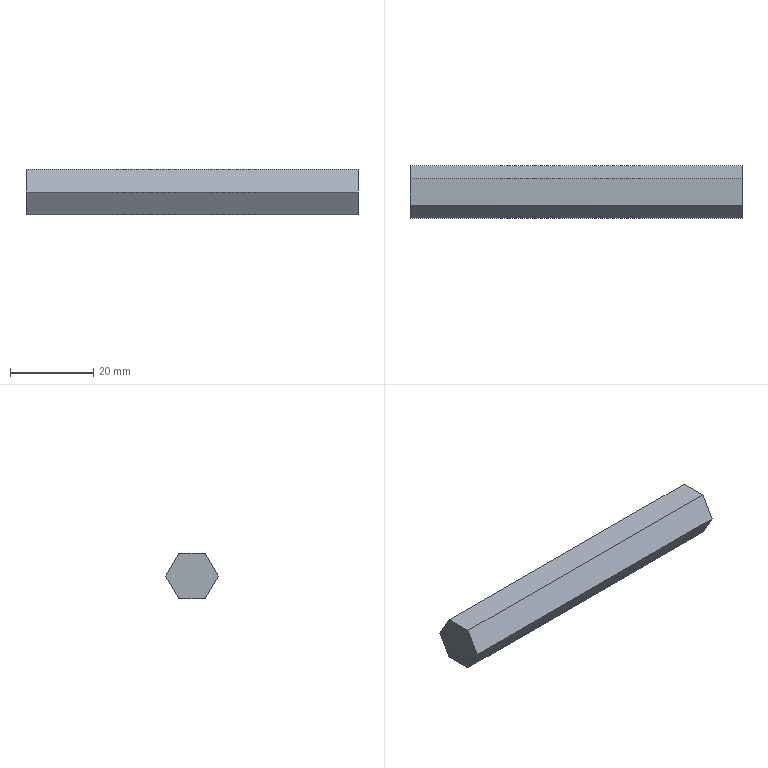Part | NX | features BREP 1 | 1 solid | 8 faces | box 80 x 12.702 x 11 mm | volume 8383 mm3 | plane 8
STEP:
#1=CARTESIAN_POINT('',(0.,-3.175,-5.5));
#2=VERTEX_POINT('',#1);
#3=CARTESIAN_POINT('',(0.,3.175,-5.5));
#4=VERTEX_POINT('',#3);
#5=CARTESIAN_POINT('',(0.,-3.175,-5.5));
#6=DIRECTION('',(0.,1.,0.));
#7=VECTOR('',#6,1000.);
#8=LINE('',#5,#7);
#9=EDGE_CURVE('',#2,#4,#8,.T.);
#10=ORIENTED_EDGE('',*,*,#9,.F.);
#11=CARTESIAN_POINT('',(0.,-6.351,0.));
#12=VERTEX_POINT('',#11);
#13=CARTESIAN_POINT('',(0.,-6.351,0.));
#14=DIRECTION('',(0.,0.5,-0.866));
#15=VECTOR('',#14,1000.);
#16=LINE('',#13,#15);
#17=EDGE_CURVE('',#12,#2,#16,.T.);
#18=ORIENTED_EDGE('',*,*,#17,.F.);
#19=CARTESIAN_POINT('',(0.,-3.175,5.5));
#20=VERTEX_POINT('',#19);
#21=CARTESIAN_POINT('',(0.,-3.175,5.5));
#22=DIRECTION('',(0.,-0.5,-0.866));
#23=VECTOR('',#22,1000.);
#24=LINE('',#21,#23);
#25=EDGE_CURVE('',#20,#12,#24,.T.);
#26=ORIENTED_EDGE('',*,*,#25,.F.);
#27=CARTESIAN_POINT('',(0.,3.175,5.5));
#28=VERTEX_POINT('',#27);
#29=CARTESIAN_POINT('',(0.,3.175,5.5));
#30=DIRECTION('',(0.,-1.,0.));
#31=VECTOR('',#30,1000.);
#32=LINE('',#29,#31);
#33=EDGE_CURVE('',#28,#20,#32,.T.);
#34=ORIENTED_EDGE('',*,*,#33,.F.);
#35=CARTESIAN_POINT('',(0.,6.351,0.));
#36=VERTEX_POINT('',#35);
#37=CARTESIAN_POINT('',(0.,6.351,0.));
#38=DIRECTION('',(0.,-0.5,0.866));
#39=VECTOR('',#38,1000.);
#40=LINE('',#37,#39);
#41=EDGE_CURVE('',#36,#28,#40,.T.);
#42=ORIENTED_EDGE('',*,*,#41,.F.);
#43=CARTESIAN_POINT('',(0.,3.175,-5.5));
#44=DIRECTION('',(0.,0.5,0.866));
#45=VECTOR('',#44,1000.);
#46=LINE('',#43,#45);
#47=EDGE_CURVE('',#4,#36,#46,.T.);
#48=ORIENTED_EDGE('',*,*,#47,.F.);
#49=EDGE_LOOP('',(#10,#18,#26,#34,#42,#48));
#50=FACE_BOUND('',#49,.T.);
#51=CARTESIAN_POINT('',(0.,0.,0.));
#52=DIRECTION('',(1.,0.,0.));
#53=DIRECTION('',(0.,1.,0.));
#54=AXIS2_PLACEMENT_3D('',#51,#52,#53);
#55=PLANE('',#54);
#56=ADVANCED_FACE('',(#50),#55,.F.);
#57=CARTESIAN_POINT('',(80.,6.351,0.));
#58=VERTEX_POINT('',#57);
#59=CARTESIAN_POINT('',(0.,6.351,0.));
#60=DIRECTION('',(1.,0.,0.));
#61=VECTOR('',#60,1000.);
#62=LINE('',#59,#61);
#63=EDGE_CURVE('',#36,#58,#62,.T.);
#64=ORIENTED_EDGE('',*,*,#63,.T.);
#65=CARTESIAN_POINT('',(80.,3.175,-5.5));
#66=VERTEX_POINT('',#65);
#67=CARTESIAN_POINT('',(80.,3.175,-5.5));
#68=DIRECTION('',(0.,0.5,0.866));
#69=VECTOR('',#68,1000.);
#70=LINE('',#67,#69);
#71=EDGE_CURVE('',#66,#58,#70,.T.);
#72=ORIENTED_EDGE('',*,*,#71,.F.);
#73=CARTESIAN_POINT('',(0.,3.175,-5.5));
#74=DIRECTION('',(1.,0.,0.));
#75=VECTOR('',#74,1000.);
#76=LINE('',#73,#75);
#77=EDGE_CURVE('',#4,#66,#76,.T.);
#78=ORIENTED_EDGE('',*,*,#77,.F.);
#79=ORIENTED_EDGE('',*,*,#47,.T.);
#80=EDGE_LOOP('',(#64,#72,#78,#79));
#81=FACE_BOUND('',#80,.T.);
#82=CARTESIAN_POINT('',(0.,3.175,-5.5));
#83=DIRECTION('',(0.,0.866,-0.5));
#84=DIRECTION('',(-1.,0.,0.));
#85=AXIS2_PLACEMENT_3D('',#82,#83,#84);
#86=PLANE('',#85);
#87=ADVANCED_FACE('',(#81),#86,.T.);
#88=ORIENTED_EDGE('',*,*,#77,.T.);
#89=CARTESIAN_POINT('',(80.,-3.175,-5.5));
#90=VERTEX_POINT('',#89);
#91=CARTESIAN_POINT('',(80.,-3.175,-5.5));
#92=DIRECTION('',(0.,1.,0.));
#93=VECTOR('',#92,1000.);
#94=LINE('',#91,#93);
#95=EDGE_CURVE('',#90,#66,#94,.T.);
#96=ORIENTED_EDGE('',*,*,#95,.F.);
#97=CARTESIAN_POINT('',(0.,-3.175,-5.5));
#98=DIRECTION('',(1.,0.,0.));
#99=VECTOR('',#98,1000.);
#100=LINE('',#97,#99);
#101=EDGE_CURVE('',#2,#90,#100,.T.);
#102=ORIENTED_EDGE('',*,*,#101,.F.);
#103=ORIENTED_EDGE('',*,*,#9,.T.);
#104=EDGE_LOOP('',(#88,#96,#102,#103));
#105=FACE_BOUND('',#104,.T.);
#106=CARTESIAN_POINT('',(0.,-3.175,-5.5));
#107=DIRECTION('',(0.,0.,-1.));
#108=DIRECTION('',(0.,-1.,0.));
#109=AXIS2_PLACEMENT_3D('',#106,#107,#108);
#110=PLANE('',#109);
#111=ADVANCED_FACE('',(#105),#110,.T.);
#112=ORIENTED_EDGE('',*,*,#101,.T.);
#113=CARTESIAN_POINT('',(80.,-6.351,0.));
#114=VERTEX_POINT('',#113);
#115=CARTESIAN_POINT('',(80.,-6.351,0.));
#116=DIRECTION('',(0.,0.5,-0.866));
#117=VECTOR('',#116,1000.);
#118=LINE('',#115,#117);
#119=EDGE_CURVE('',#114,#90,#118,.T.);
#120=ORIENTED_EDGE('',*,*,#119,.F.);
#121=CARTESIAN_POINT('',(0.,-6.351,0.));
#122=DIRECTION('',(1.,0.,0.));
#123=VECTOR('',#122,1000.);
#124=LINE('',#121,#123);
#125=EDGE_CURVE('',#12,#114,#124,.T.);
#126=ORIENTED_EDGE('',*,*,#125,.F.);
#127=ORIENTED_EDGE('',*,*,#17,.T.);
#128=EDGE_LOOP('',(#112,#120,#126,#127));
#129=FACE_BOUND('',#128,.T.);
#130=CARTESIAN_POINT('',(0.,-6.351,0.));
#131=DIRECTION('',(0.,-0.866,-0.5));
#132=DIRECTION('',(0.,0.5,-0.866));
#133=AXIS2_PLACEMENT_3D('',#130,#131,#132);
#134=PLANE('',#133);
#135=ADVANCED_FACE('',(#129),#134,.T.);
#136=ORIENTED_EDGE('',*,*,#125,.T.);
#137=CARTESIAN_POINT('',(80.,-3.175,5.5));
#138=VERTEX_POINT('',#137);
#139=CARTESIAN_POINT('',(80.,-3.175,5.5));
#140=DIRECTION('',(0.,-0.5,-0.866));
#141=VECTOR('',#140,1000.);
#142=LINE('',#139,#141);
#143=EDGE_CURVE('',#138,#114,#142,.T.);
#144=ORIENTED_EDGE('',*,*,#143,.F.);
#145=CARTESIAN_POINT('',(0.,-3.175,5.5));
#146=DIRECTION('',(1.,0.,0.));
#147=VECTOR('',#146,1000.);
#148=LINE('',#145,#147);
#149=EDGE_CURVE('',#20,#138,#148,.T.);
#150=ORIENTED_EDGE('',*,*,#149,.F.);
#151=ORIENTED_EDGE('',*,*,#25,.T.);
#152=EDGE_LOOP('',(#136,#144,#150,#151));
#153=FACE_BOUND('',#152,.T.);
#154=CARTESIAN_POINT('',(0.,-3.175,5.5));
#155=DIRECTION('',(0.,-0.866,0.5));
#156=DIRECTION('',(-1.,0.,0.));
#157=AXIS2_PLACEMENT_3D('',#154,#155,#156);
#158=PLANE('',#157);
#159=ADVANCED_FACE('',(#153),#158,.T.);
#160=ORIENTED_EDGE('',*,*,#149,.T.);
#161=CARTESIAN_POINT('',(80.,3.175,5.5));
#162=VERTEX_POINT('',#161);
#163=CARTESIAN_POINT('',(80.,3.175,5.5));
#164=DIRECTION('',(0.,-1.,0.));
#165=VECTOR('',#164,1000.);
#166=LINE('',#163,#165);
#167=EDGE_CURVE('',#162,#138,#166,.T.);
#168=ORIENTED_EDGE('',*,*,#167,.F.);
#169=CARTESIAN_POINT('',(0.,3.175,5.5));
#170=DIRECTION('',(1.,0.,0.));
#171=VECTOR('',#170,1000.);
#172=LINE('',#169,#171);
#173=EDGE_CURVE('',#28,#162,#172,.T.);
#174=ORIENTED_EDGE('',*,*,#173,.F.);
#175=ORIENTED_EDGE('',*,*,#33,.T.);
#176=EDGE_LOOP('',(#160,#168,#174,#175));
#177=FACE_BOUND('',#176,.T.);
#178=CARTESIAN_POINT('',(0.,3.175,5.5));
#179=DIRECTION('',(0.,0.,1.));
#180=DIRECTION('',(1.,0.,0.));
#181=AXIS2_PLACEMENT_3D('',#178,#179,#180);
#182=PLANE('',#181);
#183=ADVANCED_FACE('',(#177),#182,.T.);
#184=ORIENTED_EDGE('',*,*,#173,.T.);
#185=CARTESIAN_POINT('',(80.,6.351,0.));
#186=DIRECTION('',(0.,-0.5,0.866));
#187=VECTOR('',#186,1000.);
#188=LINE('',#185,#187);
#189=EDGE_CURVE('',#58,#162,#188,.T.);
#190=ORIENTED_EDGE('',*,*,#189,.F.);
#191=ORIENTED_EDGE('',*,*,#63,.F.);
#192=ORIENTED_EDGE('',*,*,#41,.T.);
#193=EDGE_LOOP('',(#184,#190,#191,#192));
#194=FACE_BOUND('',#193,.T.);
#195=CARTESIAN_POINT('',(0.,6.351,0.));
#196=DIRECTION('',(0.,0.866,0.5));
#197=DIRECTION('',(1.,0.,0.));
#198=AXIS2_PLACEMENT_3D('',#195,#196,#197);
#199=PLANE('',#198);
#200=ADVANCED_FACE('',(#194),#199,.T.);
#201=ORIENTED_EDGE('',*,*,#189,.T.);
#202=ORIENTED_EDGE('',*,*,#167,.T.);
#203=ORIENTED_EDGE('',*,*,#143,.T.);
#204=ORIENTED_EDGE('',*,*,#119,.T.);
#205=ORIENTED_EDGE('',*,*,#95,.T.);
#206=ORIENTED_EDGE('',*,*,#71,.T.);
#207=EDGE_LOOP('',(#201,#202,#203,#204,#205,#206));
#208=FACE_BOUND('',#207,.T.);
#209=CARTESIAN_POINT('',(80.,0.,0.));
#210=DIRECTION('',(1.,0.,0.));
#211=DIRECTION('',(0.,1.,0.));
#212=AXIS2_PLACEMENT_3D('',#209,#210,#211);
#213=PLANE('',#212);
#214=ADVANCED_FACE('',(#208),#213,.T.);
#215=CLOSED_SHELL('',(#56,#87,#111,#135,#159,#183,#200,#214));
#216=MANIFOLD_SOLID_BREP('',#215);
#217=(LENGTH_UNIT()NAMED_UNIT(*)SI_UNIT(.MILLI.,.METRE.));
#218=UNCERTAINTY_MEASURE_WITH_UNIT(LENGTH_MEASURE(0.00001),#217,'','');
#219=(NAMED_UNIT(*)PLANE_ANGLE_UNIT()SI_UNIT($,.RADIAN.));
#220=(NAMED_UNIT(*)SI_UNIT($,.STERADIAN.)SOLID_ANGLE_UNIT());
#221=(GEOMETRIC_REPRESENTATION_CONTEXT(3)GLOBAL_UNCERTAINTY_ASSIGNED_CONTEXT((#218))GLOBAL_UNIT_ASSIGNED_CONTEXT((#217,#219,#220))REPRESENTATION_CONTEXT('',''));
#222=ADVANCED_BREP_SHAPE_REPRESENTATION('',(#216),#221);